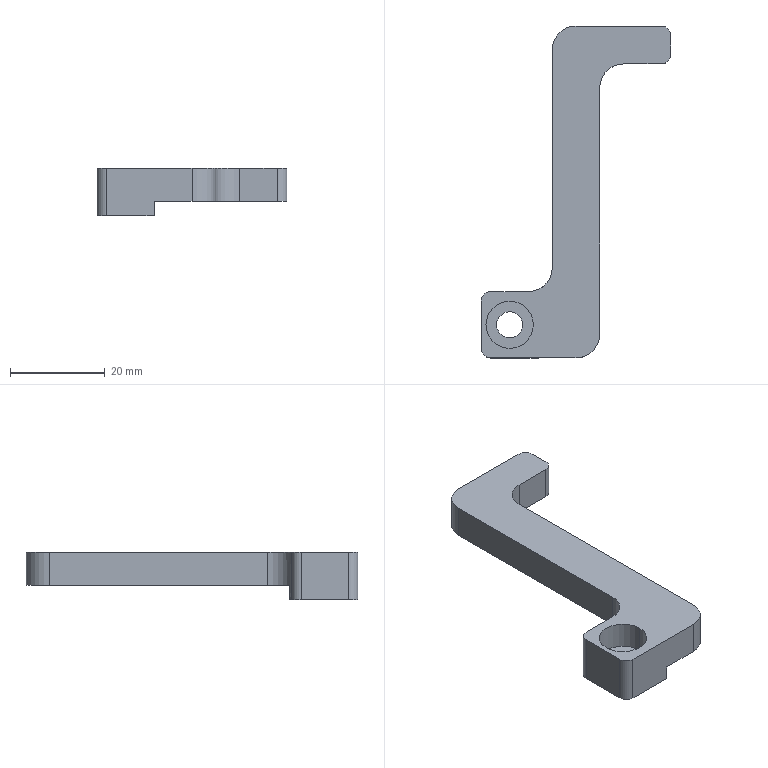Part | STEP file | FBDS-CS-027 | 1 solid | 34 faces | box 40 x 70 x 10 mm | volume 7093 mm3 | plane 18 | cylinder 16 | commonest cylinder face diameters 10 x6 4 x4 8 x4 5.5 x2
STEP:
#1=CARTESIAN_POINT('',(-14.,7.,4.3));
#2=VERTEX_POINT('',#1);
#3=CARTESIAN_POINT('',(-4.,7.,4.3));
#4=VERTEX_POINT('',#3);
#5=CARTESIAN_POINT('',(-9.,7.,4.3));
#6=DIRECTION('',(0.,0.,1.));
#7=DIRECTION('',(1.,0.,0.));
#8=AXIS2_PLACEMENT_3D('',#5,#6,#7);
#9=CIRCLE('',#8,5.);
#10=EDGE_CURVE('',#2,#4,#9,.T.);
#11=ORIENTED_EDGE('',*,*,#10,.F.);
#12=CARTESIAN_POINT('',(-14.,7.,10.));
#13=VERTEX_POINT('',#12);
#14=CARTESIAN_POINT('',(-14.,7.,10.));
#15=DIRECTION('',(0.,0.,1.));
#16=VECTOR('',#15,1000.);
#17=LINE('',#14,#16);
#18=EDGE_CURVE('',#2,#13,#17,.T.);
#19=ORIENTED_EDGE('',*,*,#18,.T.);
#20=CARTESIAN_POINT('',(-4.,7.,10.));
#21=VERTEX_POINT('',#20);
#22=CARTESIAN_POINT('',(-9.,7.,10.));
#23=DIRECTION('',(0.,0.,1.));
#24=DIRECTION('',(1.,0.,0.));
#25=AXIS2_PLACEMENT_3D('',#22,#23,#24);
#26=CIRCLE('',#25,5.);
#27=EDGE_CURVE('',#13,#21,#26,.T.);
#28=ORIENTED_EDGE('',*,*,#27,.T.);
#29=CARTESIAN_POINT('',(-4.,7.,10.));
#30=DIRECTION('',(0.,0.,1.));
#31=VECTOR('',#30,1000.);
#32=LINE('',#29,#31);
#33=EDGE_CURVE('',#4,#21,#32,.T.);
#34=ORIENTED_EDGE('',*,*,#33,.F.);
#35=EDGE_LOOP('',(#11,#19,#28,#34));
#36=FACE_OUTER_BOUND('',#35,.T.);
#37=CARTESIAN_POINT('',(-9.,7.,10.));
#38=DIRECTION('',(0.,0.,1.));
#39=DIRECTION('',(1.,0.,0.));
#40=AXIS2_PLACEMENT_3D('',#37,#38,#39);
#41=CYLINDRICAL_SURFACE('',#40,5.);
#42=ADVANCED_FACE('',(#36),#41,.F.);
#43=CARTESIAN_POINT('',(-6.25,7.,2.));
#44=VERTEX_POINT('',#43);
#45=CARTESIAN_POINT('',(-11.75,7.,2.));
#46=VERTEX_POINT('',#45);
#47=CARTESIAN_POINT('',(-9.,7.,2.));
#48=DIRECTION('',(0.,0.,-1.));
#49=DIRECTION('',(-1.,0.,0.));
#50=AXIS2_PLACEMENT_3D('',#47,#48,#49);
#51=CIRCLE('',#50,2.75);
#52=EDGE_CURVE('',#44,#46,#51,.T.);
#53=ORIENTED_EDGE('',*,*,#52,.T.);
#54=CARTESIAN_POINT('',(-11.75,7.,4.3));
#55=VERTEX_POINT('',#54);
#56=CARTESIAN_POINT('',(-11.75,7.,10.));
#57=DIRECTION('',(0.,0.,1.));
#58=VECTOR('',#57,1000.);
#59=LINE('',#56,#58);
#60=EDGE_CURVE('',#46,#55,#59,.T.);
#61=ORIENTED_EDGE('',*,*,#60,.T.);
#62=CARTESIAN_POINT('',(-6.25,7.,4.3));
#63=VERTEX_POINT('',#62);
#64=CARTESIAN_POINT('',(-9.,7.,4.3));
#65=DIRECTION('',(0.,0.,1.));
#66=DIRECTION('',(1.,0.,0.));
#67=AXIS2_PLACEMENT_3D('',#64,#65,#66);
#68=CIRCLE('',#67,2.75);
#69=EDGE_CURVE('',#55,#63,#68,.T.);
#70=ORIENTED_EDGE('',*,*,#69,.T.);
#71=CARTESIAN_POINT('',(-6.25,7.,10.));
#72=DIRECTION('',(0.,0.,1.));
#73=VECTOR('',#72,1000.);
#74=LINE('',#71,#73);
#75=EDGE_CURVE('',#44,#63,#74,.T.);
#76=ORIENTED_EDGE('',*,*,#75,.F.);
#77=EDGE_LOOP('',(#53,#61,#70,#76));
#78=FACE_OUTER_BOUND('',#77,.T.);
#79=CARTESIAN_POINT('',(-9.,7.,10.));
#80=DIRECTION('',(0.,0.,1.));
#81=DIRECTION('',(1.,0.,0.));
#82=AXIS2_PLACEMENT_3D('',#79,#80,#81);
#83=CYLINDRICAL_SURFACE('',#82,2.75);
#84=ADVANCED_FACE('',(#78),#83,.F.);
#85=CARTESIAN_POINT('',(0.,19.,3.));
#86=VERTEX_POINT('',#85);
#87=CARTESIAN_POINT('',(0.,65.,3.));
#88=VERTEX_POINT('',#87);
#89=CARTESIAN_POINT('',(0.,70.,3.));
#90=DIRECTION('',(0.,1.,0.));
#91=VECTOR('',#90,1000.);
#92=LINE('',#89,#91);
#93=EDGE_CURVE('',#86,#88,#92,.T.);
#94=ORIENTED_EDGE('',*,*,#93,.F.);
#95=CARTESIAN_POINT('',(0.,19.,10.));
#96=VERTEX_POINT('',#95);
#97=CARTESIAN_POINT('',(0.,19.,10.));
#98=DIRECTION('',(0.,0.,1.));
#99=VECTOR('',#98,1000.);
#100=LINE('',#97,#99);
#101=EDGE_CURVE('',#86,#96,#100,.T.);
#102=ORIENTED_EDGE('',*,*,#101,.T.);
#103=CARTESIAN_POINT('',(0.,65.,10.));
#104=VERTEX_POINT('',#103);
#105=CARTESIAN_POINT('',(0.,70.,10.));
#106=DIRECTION('',(0.,-1.,0.));
#107=VECTOR('',#106,1000.);
#108=LINE('',#105,#107);
#109=EDGE_CURVE('',#104,#96,#108,.T.);
#110=ORIENTED_EDGE('',*,*,#109,.F.);
#111=CARTESIAN_POINT('',(0.,65.,10.));
#112=DIRECTION('',(0.,0.,-1.));
#113=VECTOR('',#112,1000.);
#114=LINE('',#111,#113);
#115=EDGE_CURVE('',#104,#88,#114,.T.);
#116=ORIENTED_EDGE('',*,*,#115,.T.);
#117=EDGE_LOOP('',(#94,#102,#110,#116));
#118=FACE_OUTER_BOUND('',#117,.T.);
#119=CARTESIAN_POINT('',(0.,70.,10.));
#120=DIRECTION('',(1.,0.,0.));
#121=DIRECTION('',(0.,1.,0.));
#122=AXIS2_PLACEMENT_3D('',#119,#120,#121);
#123=PLANE('',#122);
#124=ADVANCED_FACE('',(#118),#123,.F.);
#125=CARTESIAN_POINT('',(10.,57.,3.));
#126=VERTEX_POINT('',#125);
#127=CARTESIAN_POINT('',(10.,5.,3.));
#128=VERTEX_POINT('',#127);
#129=CARTESIAN_POINT('',(10.,0.,3.));
#130=DIRECTION('',(0.,-1.,0.));
#131=VECTOR('',#130,1000.);
#132=LINE('',#129,#131);
#133=EDGE_CURVE('',#126,#128,#132,.T.);
#134=ORIENTED_EDGE('',*,*,#133,.F.);
#135=CARTESIAN_POINT('',(10.,57.,10.));
#136=VERTEX_POINT('',#135);
#137=CARTESIAN_POINT('',(10.,57.,10.));
#138=DIRECTION('',(0.,0.,1.));
#139=VECTOR('',#138,1000.);
#140=LINE('',#137,#139);
#141=EDGE_CURVE('',#126,#136,#140,.T.);
#142=ORIENTED_EDGE('',*,*,#141,.T.);
#143=CARTESIAN_POINT('',(10.,5.,10.));
#144=VERTEX_POINT('',#143);
#145=CARTESIAN_POINT('',(10.,0.,10.));
#146=DIRECTION('',(0.,1.,0.));
#147=VECTOR('',#146,1000.);
#148=LINE('',#145,#147);
#149=EDGE_CURVE('',#144,#136,#148,.T.);
#150=ORIENTED_EDGE('',*,*,#149,.F.);
#151=CARTESIAN_POINT('',(10.,5.,10.));
#152=DIRECTION('',(0.,0.,-1.));
#153=VECTOR('',#152,1000.);
#154=LINE('',#151,#153);
#155=EDGE_CURVE('',#144,#128,#154,.T.);
#156=ORIENTED_EDGE('',*,*,#155,.T.);
#157=EDGE_LOOP('',(#134,#142,#150,#156));
#158=FACE_OUTER_BOUND('',#157,.T.);
#159=CARTESIAN_POINT('',(10.,0.,10.));
#160=DIRECTION('',(-1.,0.,0.));
#161=DIRECTION('',(0.,0.,1.));
#162=AXIS2_PLACEMENT_3D('',#159,#160,#161);
#163=PLANE('',#162);
#164=ADVANCED_FACE('',(#158),#163,.F.);
#165=CARTESIAN_POINT('',(23.,62.,3.));
#166=VERTEX_POINT('',#165);
#167=CARTESIAN_POINT('',(15.,62.,3.));
#168=VERTEX_POINT('',#167);
#169=CARTESIAN_POINT('',(10.,62.,3.));
#170=DIRECTION('',(-1.,0.,0.));
#171=VECTOR('',#170,1000.);
#172=LINE('',#169,#171);
#173=EDGE_CURVE('',#166,#168,#172,.T.);
#174=ORIENTED_EDGE('',*,*,#173,.F.);
#175=CARTESIAN_POINT('',(23.,62.,10.));
#176=VERTEX_POINT('',#175);
#177=CARTESIAN_POINT('',(23.,62.,10.));
#178=DIRECTION('',(0.,0.,1.));
#179=VECTOR('',#178,1000.);
#180=LINE('',#177,#179);
#181=EDGE_CURVE('',#166,#176,#180,.T.);
#182=ORIENTED_EDGE('',*,*,#181,.T.);
#183=CARTESIAN_POINT('',(15.,62.,10.));
#184=VERTEX_POINT('',#183);
#185=CARTESIAN_POINT('',(10.,62.,10.));
#186=DIRECTION('',(1.,0.,0.));
#187=VECTOR('',#186,1000.);
#188=LINE('',#185,#187);
#189=EDGE_CURVE('',#184,#176,#188,.T.);
#190=ORIENTED_EDGE('',*,*,#189,.F.);
#191=CARTESIAN_POINT('',(15.,62.,0.));
#192=DIRECTION('',(0.,0.,-1.));
#193=VECTOR('',#192,1000.);
#194=LINE('',#191,#193);
#195=EDGE_CURVE('',#184,#168,#194,.T.);
#196=ORIENTED_EDGE('',*,*,#195,.T.);
#197=EDGE_LOOP('',(#174,#182,#190,#196));
#198=FACE_OUTER_BOUND('',#197,.T.);
#199=CARTESIAN_POINT('',(10.,62.,10.));
#200=DIRECTION('',(0.,1.,0.));
#201=DIRECTION('',(0.,0.,1.));
#202=AXIS2_PLACEMENT_3D('',#199,#200,#201);
#203=PLANE('',#202);
#204=ADVANCED_FACE('',(#198),#203,.F.);
#205=CARTESIAN_POINT('',(25.,64.,10.));
#206=VERTEX_POINT('',#205);
#207=CARTESIAN_POINT('',(25.,68.,10.));
#208=VERTEX_POINT('',#207);
#209=CARTESIAN_POINT('',(25.,62.,10.));
#210=DIRECTION('',(0.,1.,0.));
#211=VECTOR('',#210,1000.);
#212=LINE('',#209,#211);
#213=EDGE_CURVE('',#206,#208,#212,.T.);
#214=ORIENTED_EDGE('',*,*,#213,.F.);
#215=CARTESIAN_POINT('',(25.,64.,3.));
#216=VERTEX_POINT('',#215);
#217=CARTESIAN_POINT('',(25.,64.,10.));
#218=DIRECTION('',(0.,0.,-1.));
#219=VECTOR('',#218,1000.);
#220=LINE('',#217,#219);
#221=EDGE_CURVE('',#206,#216,#220,.T.);
#222=ORIENTED_EDGE('',*,*,#221,.T.);
#223=CARTESIAN_POINT('',(25.,68.,3.));
#224=VERTEX_POINT('',#223);
#225=CARTESIAN_POINT('',(25.,70.,3.));
#226=DIRECTION('',(0.,-1.,0.));
#227=VECTOR('',#226,1000.);
#228=LINE('',#225,#227);
#229=EDGE_CURVE('',#224,#216,#228,.T.);
#230=ORIENTED_EDGE('',*,*,#229,.F.);
#231=CARTESIAN_POINT('',(25.,68.,10.));
#232=DIRECTION('',(0.,0.,1.));
#233=VECTOR('',#232,1000.);
#234=LINE('',#231,#233);
#235=EDGE_CURVE('',#224,#208,#234,.T.);
#236=ORIENTED_EDGE('',*,*,#235,.T.);
#237=EDGE_LOOP('',(#214,#222,#230,#236));
#238=FACE_OUTER_BOUND('',#237,.T.);
#239=CARTESIAN_POINT('',(25.,62.,10.));
#240=DIRECTION('',(-1.,0.,0.));
#241=DIRECTION('',(0.,0.,1.));
#242=AXIS2_PLACEMENT_3D('',#239,#240,#241);
#243=PLANE('',#242);
#244=ADVANCED_FACE('',(#238),#243,.F.);
#245=CARTESIAN_POINT('',(23.,70.,10.));
#246=VERTEX_POINT('',#245);
#247=CARTESIAN_POINT('',(5.,70.,10.));
#248=VERTEX_POINT('',#247);
#249=CARTESIAN_POINT('',(25.,70.,10.));
#250=DIRECTION('',(-1.,0.,0.));
#251=VECTOR('',#250,1000.);
#252=LINE('',#249,#251);
#253=EDGE_CURVE('',#246,#248,#252,.T.);
#254=ORIENTED_EDGE('',*,*,#253,.F.);
#255=CARTESIAN_POINT('',(23.,70.,3.));
#256=VERTEX_POINT('',#255);
#257=CARTESIAN_POINT('',(23.,70.,10.));
#258=DIRECTION('',(0.,0.,-1.));
#259=VECTOR('',#258,1000.);
#260=LINE('',#257,#259);
#261=EDGE_CURVE('',#246,#256,#260,.T.);
#262=ORIENTED_EDGE('',*,*,#261,.T.);
#263=CARTESIAN_POINT('',(5.,70.,3.));
#264=VERTEX_POINT('',#263);
#265=CARTESIAN_POINT('',(25.,70.,3.));
#266=DIRECTION('',(1.,0.,0.));
#267=VECTOR('',#266,1000.);
#268=LINE('',#265,#267);
#269=EDGE_CURVE('',#264,#256,#268,.T.);
#270=ORIENTED_EDGE('',*,*,#269,.F.);
#271=CARTESIAN_POINT('',(5.,70.,10.));
#272=DIRECTION('',(0.,0.,1.));
#273=VECTOR('',#272,1000.);
#274=LINE('',#271,#273);
#275=EDGE_CURVE('',#264,#248,#274,.T.);
#276=ORIENTED_EDGE('',*,*,#275,.T.);
#277=EDGE_LOOP('',(#254,#262,#270,#276));
#278=FACE_OUTER_BOUND('',#277,.T.);
#279=CARTESIAN_POINT('',(25.,70.,10.));
#280=DIRECTION('',(0.,-1.,0.));
#281=DIRECTION('',(0.,0.,-1.));
#282=AXIS2_PLACEMENT_3D('',#279,#280,#281);
#283=PLANE('',#282);
#284=ADVANCED_FACE('',(#278),#283,.F.);
#285=ORIENTED_EDGE('',*,*,#275,.F.);
#286=CARTESIAN_POINT('',(5.,65.,3.));
#287=DIRECTION('',(0.,0.,1.));
#288=DIRECTION('',(-1.,0.,0.));
#289=AXIS2_PLACEMENT_3D('',#286,#287,#288);
#290=CIRCLE('',#289,5.);
#291=EDGE_CURVE('',#264,#88,#290,.T.);
#292=ORIENTED_EDGE('',*,*,#291,.T.);
#293=ORIENTED_EDGE('',*,*,#115,.F.);
#294=CARTESIAN_POINT('',(5.,65.,10.));
#295=DIRECTION('',(0.,0.,1.));
#296=DIRECTION('',(1.,0.,0.));
#297=AXIS2_PLACEMENT_3D('',#294,#295,#296);
#298=CIRCLE('',#297,5.);
#299=EDGE_CURVE('',#248,#104,#298,.T.);
#300=ORIENTED_EDGE('',*,*,#299,.F.);
#301=EDGE_LOOP('',(#285,#292,#293,#300));
#302=FACE_OUTER_BOUND('',#301,.T.);
#303=CARTESIAN_POINT('',(5.,65.,10.));
#304=DIRECTION('',(0.,0.,-1.));
#305=DIRECTION('',(-1.,0.,0.));
#306=AXIS2_PLACEMENT_3D('',#303,#304,#305);
#307=CYLINDRICAL_SURFACE('',#306,5.);
#308=ADVANCED_FACE('',(#302),#307,.T.);
#309=CARTESIAN_POINT('',(5.,0.,3.));
#310=VERTEX_POINT('',#309);
#311=CARTESIAN_POINT('',(5.,0.,10.));
#312=VERTEX_POINT('',#311);
#313=CARTESIAN_POINT('',(5.,0.,10.));
#314=DIRECTION('',(0.,0.,1.));
#315=VECTOR('',#314,1000.);
#316=LINE('',#313,#315);
#317=EDGE_CURVE('',#310,#312,#316,.T.);
#318=ORIENTED_EDGE('',*,*,#317,.F.);
#319=CARTESIAN_POINT('',(5.,5.,3.));
#320=DIRECTION('',(0.,0.,1.));
#321=DIRECTION('',(-1.,0.,0.));
#322=AXIS2_PLACEMENT_3D('',#319,#320,#321);
#323=CIRCLE('',#322,5.);
#324=EDGE_CURVE('',#310,#128,#323,.T.);
#325=ORIENTED_EDGE('',*,*,#324,.T.);
#326=ORIENTED_EDGE('',*,*,#155,.F.);
#327=CARTESIAN_POINT('',(5.,5.,10.));
#328=DIRECTION('',(0.,0.,1.));
#329=DIRECTION('',(1.,0.,0.));
#330=AXIS2_PLACEMENT_3D('',#327,#328,#329);
#331=CIRCLE('',#330,5.);
#332=EDGE_CURVE('',#312,#144,#331,.T.);
#333=ORIENTED_EDGE('',*,*,#332,.F.);
#334=EDGE_LOOP('',(#318,#325,#326,#333));
#335=FACE_OUTER_BOUND('',#334,.T.);
#336=CARTESIAN_POINT('',(5.,5.,10.));
#337=DIRECTION('',(0.,0.,-1.));
#338=DIRECTION('',(-1.,0.,0.));
#339=AXIS2_PLACEMENT_3D('',#336,#337,#338);
#340=CYLINDRICAL_SURFACE('',#339,5.);
#341=ADVANCED_FACE('',(#335),#340,.T.);
#342=CARTESIAN_POINT('',(15.,57.,3.));
#343=DIRECTION('',(0.,0.,1.));
#344=DIRECTION('',(-1.,0.,0.));
#345=AXIS2_PLACEMENT_3D('',#342,#343,#344);
#346=CIRCLE('',#345,5.);
#347=EDGE_CURVE('',#168,#126,#346,.T.);
#348=ORIENTED_EDGE('',*,*,#347,.F.);
#349=ORIENTED_EDGE('',*,*,#195,.F.);
#350=CARTESIAN_POINT('',(15.,57.,10.));
#351=DIRECTION('',(0.,0.,-1.));
#352=DIRECTION('',(1.,0.,0.));
#353=AXIS2_PLACEMENT_3D('',#350,#351,#352);
#354=CIRCLE('',#353,5.);
#355=EDGE_CURVE('',#136,#184,#354,.T.);
#356=ORIENTED_EDGE('',*,*,#355,.F.);
#357=ORIENTED_EDGE('',*,*,#141,.F.);
#358=EDGE_LOOP('',(#348,#349,#356,#357));
#359=FACE_OUTER_BOUND('',#358,.T.);
#360=CARTESIAN_POINT('',(15.,57.,10.));
#361=DIRECTION('',(0.,0.,1.));
#362=DIRECTION('',(1.,0.,0.));
#363=AXIS2_PLACEMENT_3D('',#360,#361,#362);
#364=CYLINDRICAL_SURFACE('',#363,5.);
#365=ADVANCED_FACE('',(#359),#364,.F.);
#366=CARTESIAN_POINT('',(-13.,0.,10.));
#367=VERTEX_POINT('',#366);
#368=CARTESIAN_POINT('',(0.,0.,10.));
#369=DIRECTION('',(1.,0.,0.));
#370=VECTOR('',#369,1000.);
#371=LINE('',#368,#370);
#372=EDGE_CURVE('',#367,#312,#371,.T.);
#373=ORIENTED_EDGE('',*,*,#372,.F.);
#374=CARTESIAN_POINT('',(-13.,0.,0.));
#375=VERTEX_POINT('',#374);
#376=CARTESIAN_POINT('',(-13.,0.,0.));
#377=DIRECTION('',(0.,0.,-1.));
#378=VECTOR('',#377,1000.);
#379=LINE('',#376,#378);
#380=EDGE_CURVE('',#367,#375,#379,.T.);
#381=ORIENTED_EDGE('',*,*,#380,.T.);
#382=CARTESIAN_POINT('',(-3.,0.,0.));
#383=VERTEX_POINT('',#382);
#384=CARTESIAN_POINT('',(0.,0.,0.));
#385=DIRECTION('',(1.,0.,0.));
#386=VECTOR('',#385,1000.);
#387=LINE('',#384,#386);
#388=EDGE_CURVE('',#375,#383,#387,.T.);
#389=ORIENTED_EDGE('',*,*,#388,.T.);
#390=CARTESIAN_POINT('',(-3.,0.,3.));
#391=VERTEX_POINT('',#390);
#392=CARTESIAN_POINT('',(-3.,0.,10.));
#393=DIRECTION('',(0.,0.,1.));
#394=VECTOR('',#393,1000.);
#395=LINE('',#392,#394);
#396=EDGE_CURVE('',#383,#391,#395,.T.);
#397=ORIENTED_EDGE('',*,*,#396,.T.);
#398=CARTESIAN_POINT('',(0.,0.,3.));
#399=DIRECTION('',(-1.,0.,0.));
#400=VECTOR('',#399,1000.);
#401=LINE('',#398,#400);
#402=EDGE_CURVE('',#310,#391,#401,.T.);
#403=ORIENTED_EDGE('',*,*,#402,.F.);
#404=ORIENTED_EDGE('',*,*,#317,.T.);
#405=EDGE_LOOP('',(#373,#381,#389,#397,#403,#404));
#406=FACE_OUTER_BOUND('',#405,.T.);
#407=CARTESIAN_POINT('',(0.,0.,10.));
#408=DIRECTION('',(0.,1.,0.));
#409=DIRECTION('',(0.,0.,1.));
#410=AXIS2_PLACEMENT_3D('',#407,#408,#409);
#411=PLANE('',#410);
#412=ADVANCED_FACE('',(#406),#411,.F.);
#413=CARTESIAN_POINT('',(-9.,7.,10.));
#414=DIRECTION('',(0.,0.,1.));
#415=DIRECTION('',(1.,0.,0.));
#416=AXIS2_PLACEMENT_3D('',#413,#414,#415);
#417=CIRCLE('',#416,5.);
#418=EDGE_CURVE('',#21,#13,#417,.T.);
#419=ORIENTED_EDGE('',*,*,#418,.F.);
#420=ORIENTED_EDGE('',*,*,#27,.F.);
#421=EDGE_LOOP('',(#419,#420));
#422=FACE_BOUND('',#421,.T.);
#423=ORIENTED_EDGE('',*,*,#189,.T.);
#424=CARTESIAN_POINT('',(23.,64.,10.));
#425=DIRECTION('',(0.,0.,1.));
#426=DIRECTION('',(1.,0.,0.));
#427=AXIS2_PLACEMENT_3D('',#424,#425,#426);
#428=CIRCLE('',#427,2.);
#429=EDGE_CURVE('',#176,#206,#428,.T.);
#430=ORIENTED_EDGE('',*,*,#429,.T.);
#431=ORIENTED_EDGE('',*,*,#213,.T.);
#432=CARTESIAN_POINT('',(23.,68.,10.));
#433=DIRECTION('',(0.,0.,1.));
#434=DIRECTION('',(1.,0.,0.));
#435=AXIS2_PLACEMENT_3D('',#432,#433,#434);
#436=CIRCLE('',#435,2.);
#437=EDGE_CURVE('',#208,#246,#436,.T.);
#438=ORIENTED_EDGE('',*,*,#437,.T.);
#439=ORIENTED_EDGE('',*,*,#253,.T.);
#440=ORIENTED_EDGE('',*,*,#299,.T.);
#441=ORIENTED_EDGE('',*,*,#109,.T.);
#442=CARTESIAN_POINT('',(-5.,14.,10.));
#443=VERTEX_POINT('',#442);
#444=CARTESIAN_POINT('',(-5.,19.,10.));
#445=DIRECTION('',(0.,0.,-1.));
#446=DIRECTION('',(1.,0.,0.));
#447=AXIS2_PLACEMENT_3D('',#444,#445,#446);
#448=CIRCLE('',#447,5.);
#449=EDGE_CURVE('',#96,#443,#448,.T.);
#450=ORIENTED_EDGE('',*,*,#449,.T.);
#451=CARTESIAN_POINT('',(-13.,14.,10.));
#452=VERTEX_POINT('',#451);
#453=CARTESIAN_POINT('',(0.,14.,10.));
#454=DIRECTION('',(-1.,0.,0.));
#455=VECTOR('',#454,1000.);
#456=LINE('',#453,#455);
#457=EDGE_CURVE('',#443,#452,#456,.T.);
#458=ORIENTED_EDGE('',*,*,#457,.T.);
#459=CARTESIAN_POINT('',(-15.,12.,10.));
#460=VERTEX_POINT('',#459);
#461=CARTESIAN_POINT('',(-13.,12.,10.));
#462=DIRECTION('',(0.,0.,1.));
#463=DIRECTION('',(1.,0.,0.));
#464=AXIS2_PLACEMENT_3D('',#461,#462,#463);
#465=CIRCLE('',#464,2.);
#466=EDGE_CURVE('',#452,#460,#465,.T.);
#467=ORIENTED_EDGE('',*,*,#466,.T.);
#468=CARTESIAN_POINT('',(-15.,2.,10.));
#469=VERTEX_POINT('',#468);
#470=CARTESIAN_POINT('',(-15.,0.,10.));
#471=DIRECTION('',(0.,-1.,0.));
#472=VECTOR('',#471,1000.);
#473=LINE('',#470,#472);
#474=EDGE_CURVE('',#460,#469,#473,.T.);
#475=ORIENTED_EDGE('',*,*,#474,.T.);
#476=CARTESIAN_POINT('',(-13.,2.,10.));
#477=DIRECTION('',(0.,0.,1.));
#478=DIRECTION('',(1.,0.,0.));
#479=AXIS2_PLACEMENT_3D('',#476,#477,#478);
#480=CIRCLE('',#479,2.);
#481=EDGE_CURVE('',#469,#367,#480,.T.);
#482=ORIENTED_EDGE('',*,*,#481,.T.);
#483=ORIENTED_EDGE('',*,*,#372,.T.);
#484=ORIENTED_EDGE('',*,*,#332,.T.);
#485=ORIENTED_EDGE('',*,*,#149,.T.);
#486=ORIENTED_EDGE('',*,*,#355,.T.);
#487=EDGE_LOOP('',(#423,#430,#431,#438,#439,#440,#441,#450,#458,#467,#475,#482,#483,#484,#485,#486));
#488=FACE_OUTER_BOUND('',#487,.T.);
#489=CARTESIAN_POINT('',(0.,0.,10.));
#490=DIRECTION('',(0.,0.,1.));
#491=DIRECTION('',(1.,0.,0.));
#492=AXIS2_PLACEMENT_3D('',#489,#490,#491);
#493=PLANE('',#492);
#494=ADVANCED_FACE('',(#422,#488),#493,.T.);
#495=CARTESIAN_POINT('',(-10.936,10.5,0.));
#496=VERTEX_POINT('',#495);
#497=CARTESIAN_POINT('',(-7.064,10.5,0.));
#498=VERTEX_POINT('',#497);
#499=CARTESIAN_POINT('',(-7.064,10.5,0.));
#500=DIRECTION('',(1.,0.,0.));
#501=VECTOR('',#500,1000.);
#502=LINE('',#499,#501);
#503=EDGE_CURVE('',#496,#498,#502,.T.);
#504=ORIENTED_EDGE('',*,*,#503,.F.);
#505=CARTESIAN_POINT('',(-12.5,8.936,0.));
#506=VERTEX_POINT('',#505);
#507=CARTESIAN_POINT('',(-9.,7.,0.));
#508=DIRECTION('',(0.,0.,-1.));
#509=DIRECTION('',(-1.,0.,0.));
#510=AXIS2_PLACEMENT_3D('',#507,#508,#509);
#511=CIRCLE('',#510,4.);
#512=EDGE_CURVE('',#506,#496,#511,.T.);
#513=ORIENTED_EDGE('',*,*,#512,.F.);
#514=CARTESIAN_POINT('',(-12.5,5.064,0.));
#515=VERTEX_POINT('',#514);
#516=CARTESIAN_POINT('',(-12.5,5.064,0.));
#517=DIRECTION('',(0.,1.,0.));
#518=VECTOR('',#517,1000.);
#519=LINE('',#516,#518);
#520=EDGE_CURVE('',#515,#506,#519,.T.);
#521=ORIENTED_EDGE('',*,*,#520,.F.);
#522=CARTESIAN_POINT('',(-10.936,3.5,0.));
#523=VERTEX_POINT('',#522);
#524=CARTESIAN_POINT('',(-9.,7.,0.));
#525=DIRECTION('',(0.,0.,-1.));
#526=DIRECTION('',(-1.,0.,0.));
#527=AXIS2_PLACEMENT_3D('',#524,#525,#526);
#528=CIRCLE('',#527,4.);
#529=EDGE_CURVE('',#523,#515,#528,.T.);
#530=ORIENTED_EDGE('',*,*,#529,.F.);
#531=CARTESIAN_POINT('',(-7.064,3.5,0.));
#532=VERTEX_POINT('',#531);
#533=CARTESIAN_POINT('',(-7.064,3.5,0.));
#534=DIRECTION('',(-1.,0.,0.));
#535=VECTOR('',#534,1000.);
#536=LINE('',#533,#535);
#537=EDGE_CURVE('',#532,#523,#536,.T.);
#538=ORIENTED_EDGE('',*,*,#537,.F.);
#539=CARTESIAN_POINT('',(-5.5,5.064,0.));
#540=VERTEX_POINT('',#539);
#541=CARTESIAN_POINT('',(-9.,7.,0.));
#542=DIRECTION('',(0.,0.,-1.));
#543=DIRECTION('',(-1.,0.,0.));
#544=AXIS2_PLACEMENT_3D('',#541,#542,#543);
#545=CIRCLE('',#544,4.);
#546=EDGE_CURVE('',#540,#532,#545,.T.);
#547=ORIENTED_EDGE('',*,*,#546,.F.);
#548=CARTESIAN_POINT('',(-5.5,8.936,0.));
#549=VERTEX_POINT('',#548);
#550=CARTESIAN_POINT('',(-5.5,5.064,0.));
#551=DIRECTION('',(0.,-1.,0.));
#552=VECTOR('',#551,1000.);
#553=LINE('',#550,#552);
#554=EDGE_CURVE('',#549,#540,#553,.T.);
#555=ORIENTED_EDGE('',*,*,#554,.F.);
#556=CARTESIAN_POINT('',(-9.,7.,0.));
#557=DIRECTION('',(0.,0.,-1.));
#558=DIRECTION('',(-1.,0.,0.));
#559=AXIS2_PLACEMENT_3D('',#556,#557,#558);
#560=CIRCLE('',#559,4.);
#561=EDGE_CURVE('',#498,#549,#560,.T.);
#562=ORIENTED_EDGE('',*,*,#561,.F.);
#563=EDGE_LOOP('',(#504,#513,#521,#530,#538,#547,#555,#562));
#564=FACE_BOUND('',#563,.T.);
#565=ORIENTED_EDGE('',*,*,#388,.F.);
#566=CARTESIAN_POINT('',(-15.,2.,0.));
#567=VERTEX_POINT('',#566);
#568=CARTESIAN_POINT('',(-13.,2.,0.));
#569=DIRECTION('',(0.,0.,-1.));
#570=DIRECTION('',(1.,0.,0.));
#571=AXIS2_PLACEMENT_3D('',#568,#569,#570);
#572=CIRCLE('',#571,2.);
#573=EDGE_CURVE('',#375,#567,#572,.T.);
#574=ORIENTED_EDGE('',*,*,#573,.T.);
#575=CARTESIAN_POINT('',(-15.,12.,0.));
#576=VERTEX_POINT('',#575);
#577=CARTESIAN_POINT('',(-15.,0.,0.));
#578=DIRECTION('',(0.,1.,0.));
#579=VECTOR('',#578,1000.);
#580=LINE('',#577,#579);
#581=EDGE_CURVE('',#567,#576,#580,.T.);
#582=ORIENTED_EDGE('',*,*,#581,.T.);
#583=CARTESIAN_POINT('',(-13.,14.,0.));
#584=VERTEX_POINT('',#583);
#585=CARTESIAN_POINT('',(-13.,12.,0.));
#586=DIRECTION('',(0.,0.,-1.));
#587=DIRECTION('',(1.,0.,0.));
#588=AXIS2_PLACEMENT_3D('',#585,#586,#587);
#589=CIRCLE('',#588,2.);
#590=EDGE_CURVE('',#576,#584,#589,.T.);
#591=ORIENTED_EDGE('',*,*,#590,.T.);
#592=CARTESIAN_POINT('',(-5.,14.,0.));
#593=VERTEX_POINT('',#592);
#594=CARTESIAN_POINT('',(0.,14.,0.));
#595=DIRECTION('',(1.,0.,0.));
#596=VECTOR('',#595,1000.);
#597=LINE('',#594,#596);
#598=EDGE_CURVE('',#584,#593,#597,.T.);
#599=ORIENTED_EDGE('',*,*,#598,.T.);
#600=CARTESIAN_POINT('',(-3.,14.417,0.));
#601=VERTEX_POINT('',#600);
#602=CARTESIAN_POINT('',(-5.,19.,0.));
#603=DIRECTION('',(0.,0.,1.));
#604=DIRECTION('',(1.,0.,0.));
#605=AXIS2_PLACEMENT_3D('',#602,#603,#604);
#606=CIRCLE('',#605,5.);
#607=EDGE_CURVE('',#593,#601,#606,.T.);
#608=ORIENTED_EDGE('',*,*,#607,.T.);
#609=CARTESIAN_POINT('',(-3.,70.,0.));
#610=DIRECTION('',(0.,1.,0.));
#611=VECTOR('',#610,1000.);
#612=LINE('',#609,#611);
#613=EDGE_CURVE('',#383,#601,#612,.T.);
#614=ORIENTED_EDGE('',*,*,#613,.F.);
#615=EDGE_LOOP('',(#565,#574,#582,#591,#599,#608,#614));
#616=FACE_OUTER_BOUND('',#615,.T.);
#617=CARTESIAN_POINT('',(0.,0.,0.));
#618=DIRECTION('',(0.,0.,1.));
#619=DIRECTION('',(1.,0.,0.));
#620=AXIS2_PLACEMENT_3D('',#617,#618,#619);
#621=PLANE('',#620);
#622=ADVANCED_FACE('',(#564,#616),#621,.F.);
#623=ORIENTED_EDGE('',*,*,#581,.F.);
#624=CARTESIAN_POINT('',(-15.,2.,10.));
#625=DIRECTION('',(0.,0.,1.));
#626=VECTOR('',#625,1000.);
#627=LINE('',#624,#626);
#628=EDGE_CURVE('',#567,#469,#627,.T.);
#629=ORIENTED_EDGE('',*,*,#628,.T.);
#630=ORIENTED_EDGE('',*,*,#474,.F.);
#631=CARTESIAN_POINT('',(-15.,12.,-20.518));
#632=DIRECTION('',(0.,0.,-1.));
#633=VECTOR('',#632,1000.);
#634=LINE('',#631,#633);
#635=EDGE_CURVE('',#460,#576,#634,.T.);
#636=ORIENTED_EDGE('',*,*,#635,.T.);
#637=EDGE_LOOP('',(#623,#629,#630,#636));
#638=FACE_OUTER_BOUND('',#637,.T.);
#639=CARTESIAN_POINT('',(-15.,0.,-20.518));
#640=DIRECTION('',(-1.,0.,0.));
#641=DIRECTION('',(0.,0.,1.));
#642=AXIS2_PLACEMENT_3D('',#639,#640,#641);
#643=PLANE('',#642);
#644=ADVANCED_FACE('',(#638),#643,.T.);
#645=ORIENTED_EDGE('',*,*,#598,.F.);
#646=CARTESIAN_POINT('',(-13.,14.,-20.518));
#647=DIRECTION('',(0.,0.,1.));
#648=VECTOR('',#647,1000.);
#649=LINE('',#646,#648);
#650=EDGE_CURVE('',#584,#452,#649,.T.);
#651=ORIENTED_EDGE('',*,*,#650,.T.);
#652=ORIENTED_EDGE('',*,*,#457,.F.);
#653=CARTESIAN_POINT('',(-5.,14.,-20.518));
#654=DIRECTION('',(0.,0.,-1.));
#655=VECTOR('',#654,1000.);
#656=LINE('',#653,#655);
#657=EDGE_CURVE('',#443,#593,#656,.T.);
#658=ORIENTED_EDGE('',*,*,#657,.T.);
#659=EDGE_LOOP('',(#645,#651,#652,#658));
#660=FACE_OUTER_BOUND('',#659,.T.);
#661=CARTESIAN_POINT('',(0.,14.,-20.518));
#662=DIRECTION('',(0.,1.,0.));
#663=DIRECTION('',(-1.,0.,0.));
#664=AXIS2_PLACEMENT_3D('',#661,#662,#663);
#665=PLANE('',#664);
#666=ADVANCED_FACE('',(#660),#665,.T.);
#667=ORIENTED_EDGE('',*,*,#512,.T.);
#668=CARTESIAN_POINT('',(-10.936,10.5,2.));
#669=VERTEX_POINT('',#668);
#670=CARTESIAN_POINT('',(-10.936,10.5,2.));
#671=DIRECTION('',(0.,0.,-1.));
#672=VECTOR('',#671,1000.);
#673=LINE('',#670,#672);
#674=EDGE_CURVE('',#669,#496,#673,.T.);
#675=ORIENTED_EDGE('',*,*,#674,.F.);
#676=CARTESIAN_POINT('',(-12.5,8.936,2.));
#677=VERTEX_POINT('',#676);
#678=CARTESIAN_POINT('',(-9.,7.,2.));
#679=DIRECTION('',(0.,0.,-1.));
#680=DIRECTION('',(-1.,0.,0.));
#681=AXIS2_PLACEMENT_3D('',#678,#679,#680);
#682=CIRCLE('',#681,4.);
#683=EDGE_CURVE('',#677,#669,#682,.T.);
#684=ORIENTED_EDGE('',*,*,#683,.F.);
#685=CARTESIAN_POINT('',(-12.5,8.936,2.));
#686=DIRECTION('',(0.,0.,-1.));
#687=VECTOR('',#686,1000.);
#688=LINE('',#685,#687);
#689=EDGE_CURVE('',#677,#506,#688,.T.);
#690=ORIENTED_EDGE('',*,*,#689,.T.);
#691=EDGE_LOOP('',(#667,#675,#684,#690));
#692=FACE_OUTER_BOUND('',#691,.T.);
#693=CARTESIAN_POINT('',(-9.,7.,2.));
#694=DIRECTION('',(0.,0.,-1.));
#695=DIRECTION('',(-1.,0.,0.));
#696=AXIS2_PLACEMENT_3D('',#693,#694,#695);
#697=CYLINDRICAL_SURFACE('',#696,4.);
#698=ADVANCED_FACE('',(#692),#697,.F.);
#699=ORIENTED_EDGE('',*,*,#520,.T.);
#700=ORIENTED_EDGE('',*,*,#689,.F.);
#701=CARTESIAN_POINT('',(-12.5,5.064,2.));
#702=VERTEX_POINT('',#701);
#703=CARTESIAN_POINT('',(-12.5,5.064,2.));
#704=DIRECTION('',(0.,1.,0.));
#705=VECTOR('',#704,1000.);
#706=LINE('',#703,#705);
#707=EDGE_CURVE('',#702,#677,#706,.T.);
#708=ORIENTED_EDGE('',*,*,#707,.F.);
#709=CARTESIAN_POINT('',(-12.5,5.064,2.));
#710=DIRECTION('',(0.,0.,-1.));
#711=VECTOR('',#710,1000.);
#712=LINE('',#709,#711);
#713=EDGE_CURVE('',#702,#515,#712,.T.);
#714=ORIENTED_EDGE('',*,*,#713,.T.);
#715=EDGE_LOOP('',(#699,#700,#708,#714));
#716=FACE_OUTER_BOUND('',#715,.T.);
#717=CARTESIAN_POINT('',(-12.5,5.064,2.));
#718=DIRECTION('',(-1.,0.,0.));
#719=DIRECTION('',(0.,0.,1.));
#720=AXIS2_PLACEMENT_3D('',#717,#718,#719);
#721=PLANE('',#720);
#722=ADVANCED_FACE('',(#716),#721,.F.);
#723=ORIENTED_EDGE('',*,*,#529,.T.);
#724=ORIENTED_EDGE('',*,*,#713,.F.);
#725=CARTESIAN_POINT('',(-10.936,3.5,2.));
#726=VERTEX_POINT('',#725);
#727=CARTESIAN_POINT('',(-9.,7.,2.));
#728=DIRECTION('',(0.,0.,-1.));
#729=DIRECTION('',(-1.,0.,0.));
#730=AXIS2_PLACEMENT_3D('',#727,#728,#729);
#731=CIRCLE('',#730,4.);
#732=EDGE_CURVE('',#726,#702,#731,.T.);
#733=ORIENTED_EDGE('',*,*,#732,.F.);
#734=CARTESIAN_POINT('',(-10.936,3.5,2.));
#735=DIRECTION('',(0.,0.,-1.));
#736=VECTOR('',#735,1000.);
#737=LINE('',#734,#736);
#738=EDGE_CURVE('',#726,#523,#737,.T.);
#739=ORIENTED_EDGE('',*,*,#738,.T.);
#740=EDGE_LOOP('',(#723,#724,#733,#739));
#741=FACE_OUTER_BOUND('',#740,.T.);
#742=CARTESIAN_POINT('',(-9.,7.,2.));
#743=DIRECTION('',(0.,0.,-1.));
#744=DIRECTION('',(-1.,0.,0.));
#745=AXIS2_PLACEMENT_3D('',#742,#743,#744);
#746=CYLINDRICAL_SURFACE('',#745,4.);
#747=ADVANCED_FACE('',(#741),#746,.F.);
#748=ORIENTED_EDGE('',*,*,#537,.T.);
#749=ORIENTED_EDGE('',*,*,#738,.F.);
#750=CARTESIAN_POINT('',(-7.064,3.5,2.));
#751=VERTEX_POINT('',#750);
#752=CARTESIAN_POINT('',(-7.064,3.5,2.));
#753=DIRECTION('',(-1.,0.,0.));
#754=VECTOR('',#753,1000.);
#755=LINE('',#752,#754);
#756=EDGE_CURVE('',#751,#726,#755,.T.);
#757=ORIENTED_EDGE('',*,*,#756,.F.);
#758=CARTESIAN_POINT('',(-7.064,3.5,2.));
#759=DIRECTION('',(0.,0.,-1.));
#760=VECTOR('',#759,1000.);
#761=LINE('',#758,#760);
#762=EDGE_CURVE('',#751,#532,#761,.T.);
#763=ORIENTED_EDGE('',*,*,#762,.T.);
#764=EDGE_LOOP('',(#748,#749,#757,#763));
#765=FACE_OUTER_BOUND('',#764,.T.);
#766=CARTESIAN_POINT('',(-7.064,3.5,2.));
#767=DIRECTION('',(0.,-1.,0.));
#768=DIRECTION('',(0.,0.,-1.));
#769=AXIS2_PLACEMENT_3D('',#766,#767,#768);
#770=PLANE('',#769);
#771=ADVANCED_FACE('',(#765),#770,.F.);
#772=ORIENTED_EDGE('',*,*,#546,.T.);
#773=ORIENTED_EDGE('',*,*,#762,.F.);
#774=CARTESIAN_POINT('',(-5.5,5.064,2.));
#775=VERTEX_POINT('',#774);
#776=CARTESIAN_POINT('',(-9.,7.,2.));
#777=DIRECTION('',(0.,0.,-1.));
#778=DIRECTION('',(-1.,0.,0.));
#779=AXIS2_PLACEMENT_3D('',#776,#777,#778);
#780=CIRCLE('',#779,4.);
#781=EDGE_CURVE('',#775,#751,#780,.T.);
#782=ORIENTED_EDGE('',*,*,#781,.F.);
#783=CARTESIAN_POINT('',(-5.5,5.064,2.));
#784=DIRECTION('',(0.,0.,-1.));
#785=VECTOR('',#784,1000.);
#786=LINE('',#783,#785);
#787=EDGE_CURVE('',#775,#540,#786,.T.);
#788=ORIENTED_EDGE('',*,*,#787,.T.);
#789=EDGE_LOOP('',(#772,#773,#782,#788));
#790=FACE_OUTER_BOUND('',#789,.T.);
#791=CARTESIAN_POINT('',(-9.,7.,2.));
#792=DIRECTION('',(0.,0.,-1.));
#793=DIRECTION('',(-1.,0.,0.));
#794=AXIS2_PLACEMENT_3D('',#791,#792,#793);
#795=CYLINDRICAL_SURFACE('',#794,4.);
#796=ADVANCED_FACE('',(#790),#795,.F.);
#797=ORIENTED_EDGE('',*,*,#554,.T.);
#798=ORIENTED_EDGE('',*,*,#787,.F.);
#799=CARTESIAN_POINT('',(-5.5,8.936,2.));
#800=VERTEX_POINT('',#799);
#801=CARTESIAN_POINT('',(-5.5,5.064,2.));
#802=DIRECTION('',(0.,-1.,0.));
#803=VECTOR('',#802,1000.);
#804=LINE('',#801,#803);
#805=EDGE_CURVE('',#800,#775,#804,.T.);
#806=ORIENTED_EDGE('',*,*,#805,.F.);
#807=CARTESIAN_POINT('',(-5.5,8.936,2.));
#808=DIRECTION('',(0.,0.,-1.));
#809=VECTOR('',#808,1000.);
#810=LINE('',#807,#809);
#811=EDGE_CURVE('',#800,#549,#810,.T.);
#812=ORIENTED_EDGE('',*,*,#811,.T.);
#813=EDGE_LOOP('',(#797,#798,#806,#812));
#814=FACE_OUTER_BOUND('',#813,.T.);
#815=CARTESIAN_POINT('',(-5.5,5.064,2.));
#816=DIRECTION('',(1.,0.,0.));
#817=DIRECTION('',(0.,0.,-1.));
#818=AXIS2_PLACEMENT_3D('',#815,#816,#817);
#819=PLANE('',#818);
#820=ADVANCED_FACE('',(#814),#819,.F.);
#821=ORIENTED_EDGE('',*,*,#561,.T.);
#822=ORIENTED_EDGE('',*,*,#811,.F.);
#823=CARTESIAN_POINT('',(-7.064,10.5,2.));
#824=VERTEX_POINT('',#823);
#825=CARTESIAN_POINT('',(-9.,7.,2.));
#826=DIRECTION('',(0.,0.,-1.));
#827=DIRECTION('',(-1.,0.,0.));
#828=AXIS2_PLACEMENT_3D('',#825,#826,#827);
#829=CIRCLE('',#828,4.);
#830=EDGE_CURVE('',#824,#800,#829,.T.);
#831=ORIENTED_EDGE('',*,*,#830,.F.);
#832=CARTESIAN_POINT('',(-7.064,10.5,2.));
#833=DIRECTION('',(0.,0.,-1.));
#834=VECTOR('',#833,1000.);
#835=LINE('',#832,#834);
#836=EDGE_CURVE('',#824,#498,#835,.T.);
#837=ORIENTED_EDGE('',*,*,#836,.T.);
#838=EDGE_LOOP('',(#821,#822,#831,#837));
#839=FACE_OUTER_BOUND('',#838,.T.);
#840=CARTESIAN_POINT('',(-9.,7.,2.));
#841=DIRECTION('',(0.,0.,-1.));
#842=DIRECTION('',(-1.,0.,0.));
#843=AXIS2_PLACEMENT_3D('',#840,#841,#842);
#844=CYLINDRICAL_SURFACE('',#843,4.);
#845=ADVANCED_FACE('',(#839),#844,.F.);
#846=ORIENTED_EDGE('',*,*,#503,.T.);
#847=ORIENTED_EDGE('',*,*,#836,.F.);
#848=CARTESIAN_POINT('',(-7.064,10.5,2.));
#849=DIRECTION('',(1.,0.,0.));
#850=VECTOR('',#849,1000.);
#851=LINE('',#848,#850);
#852=EDGE_CURVE('',#669,#824,#851,.T.);
#853=ORIENTED_EDGE('',*,*,#852,.F.);
#854=ORIENTED_EDGE('',*,*,#674,.T.);
#855=EDGE_LOOP('',(#846,#847,#853,#854));
#856=FACE_OUTER_BOUND('',#855,.T.);
#857=CARTESIAN_POINT('',(-7.064,10.5,2.));
#858=DIRECTION('',(0.,1.,0.));
#859=DIRECTION('',(0.,0.,1.));
#860=AXIS2_PLACEMENT_3D('',#857,#858,#859);
#861=PLANE('',#860);
#862=ADVANCED_FACE('',(#856),#861,.F.);
#863=ORIENTED_EDGE('',*,*,#52,.F.);
#864=CARTESIAN_POINT('',(-9.,7.,2.));
#865=DIRECTION('',(0.,0.,-1.));
#866=DIRECTION('',(-1.,0.,0.));
#867=AXIS2_PLACEMENT_3D('',#864,#865,#866);
#868=CIRCLE('',#867,2.75);
#869=EDGE_CURVE('',#46,#44,#868,.T.);
#870=ORIENTED_EDGE('',*,*,#869,.F.);
#871=EDGE_LOOP('',(#863,#870));
#872=FACE_BOUND('',#871,.T.);
#873=ORIENTED_EDGE('',*,*,#683,.T.);
#874=ORIENTED_EDGE('',*,*,#852,.T.);
#875=ORIENTED_EDGE('',*,*,#830,.T.);
#876=ORIENTED_EDGE('',*,*,#805,.T.);
#877=ORIENTED_EDGE('',*,*,#781,.T.);
#878=ORIENTED_EDGE('',*,*,#756,.T.);
#879=ORIENTED_EDGE('',*,*,#732,.T.);
#880=ORIENTED_EDGE('',*,*,#707,.T.);
#881=EDGE_LOOP('',(#873,#874,#875,#876,#877,#878,#879,#880));
#882=FACE_OUTER_BOUND('',#881,.T.);
#883=CARTESIAN_POINT('',(-9.,7.,2.));
#884=DIRECTION('',(0.,0.,-1.));
#885=DIRECTION('',(-1.,0.,0.));
#886=AXIS2_PLACEMENT_3D('',#883,#884,#885);
#887=PLANE('',#886);
#888=ADVANCED_FACE('',(#872,#882),#887,.T.);
#889=CARTESIAN_POINT('',(-3.,14.417,3.));
#890=VERTEX_POINT('',#889);
#891=CARTESIAN_POINT('',(-5.,19.,3.));
#892=DIRECTION('',(0.,0.,1.));
#893=DIRECTION('',(-1.,0.,0.));
#894=AXIS2_PLACEMENT_3D('',#891,#892,#893);
#895=CIRCLE('',#894,5.);
#896=EDGE_CURVE('',#890,#86,#895,.T.);
#897=ORIENTED_EDGE('',*,*,#896,.F.);
#898=CARTESIAN_POINT('',(-3.,14.417,10.));
#899=DIRECTION('',(0.,0.,-1.));
#900=VECTOR('',#899,1000.);
#901=LINE('',#898,#900);
#902=EDGE_CURVE('',#890,#601,#901,.T.);
#903=ORIENTED_EDGE('',*,*,#902,.T.);
#904=ORIENTED_EDGE('',*,*,#607,.F.);
#905=ORIENTED_EDGE('',*,*,#657,.F.);
#906=ORIENTED_EDGE('',*,*,#449,.F.);
#907=ORIENTED_EDGE('',*,*,#101,.F.);
#908=EDGE_LOOP('',(#897,#903,#904,#905,#906,#907));
#909=FACE_OUTER_BOUND('',#908,.T.);
#910=CARTESIAN_POINT('',(-5.,19.,10.));
#911=DIRECTION('',(0.,0.,1.));
#912=DIRECTION('',(1.,0.,0.));
#913=AXIS2_PLACEMENT_3D('',#910,#911,#912);
#914=CYLINDRICAL_SURFACE('',#913,5.);
#915=ADVANCED_FACE('',(#909),#914,.F.);
#916=ORIENTED_EDGE('',*,*,#60,.F.);
#917=ORIENTED_EDGE('',*,*,#869,.T.);
#918=ORIENTED_EDGE('',*,*,#75,.T.);
#919=CARTESIAN_POINT('',(-9.,7.,4.3));
#920=DIRECTION('',(0.,0.,1.));
#921=DIRECTION('',(1.,0.,0.));
#922=AXIS2_PLACEMENT_3D('',#919,#920,#921);
#923=CIRCLE('',#922,2.75);
#924=EDGE_CURVE('',#63,#55,#923,.T.);
#925=ORIENTED_EDGE('',*,*,#924,.T.);
#926=EDGE_LOOP('',(#916,#917,#918,#925));
#927=FACE_OUTER_BOUND('',#926,.T.);
#928=CARTESIAN_POINT('',(-9.,7.,10.));
#929=DIRECTION('',(0.,0.,1.));
#930=DIRECTION('',(1.,0.,0.));
#931=AXIS2_PLACEMENT_3D('',#928,#929,#930);
#932=CYLINDRICAL_SURFACE('',#931,2.75);
#933=ADVANCED_FACE('',(#927),#932,.F.);
#934=ORIENTED_EDGE('',*,*,#924,.F.);
#935=ORIENTED_EDGE('',*,*,#69,.F.);
#936=EDGE_LOOP('',(#934,#935));
#937=FACE_BOUND('',#936,.T.);
#938=CARTESIAN_POINT('',(-9.,7.,4.3));
#939=DIRECTION('',(0.,0.,1.));
#940=DIRECTION('',(1.,0.,0.));
#941=AXIS2_PLACEMENT_3D('',#938,#939,#940);
#942=CIRCLE('',#941,5.);
#943=EDGE_CURVE('',#4,#2,#942,.T.);
#944=ORIENTED_EDGE('',*,*,#943,.T.);
#945=ORIENTED_EDGE('',*,*,#10,.T.);
#946=EDGE_LOOP('',(#944,#945));
#947=FACE_OUTER_BOUND('',#946,.T.);
#948=CARTESIAN_POINT('',(-6.25,7.,4.3));
#949=DIRECTION('',(0.,0.,-1.));
#950=DIRECTION('',(-1.,0.,0.));
#951=AXIS2_PLACEMENT_3D('',#948,#949,#950);
#952=PLANE('',#951);
#953=ADVANCED_FACE('',(#937,#947),#952,.F.);
#954=ORIENTED_EDGE('',*,*,#18,.F.);
#955=ORIENTED_EDGE('',*,*,#943,.F.);
#956=ORIENTED_EDGE('',*,*,#33,.T.);
#957=ORIENTED_EDGE('',*,*,#418,.T.);
#958=EDGE_LOOP('',(#954,#955,#956,#957));
#959=FACE_OUTER_BOUND('',#958,.T.);
#960=CARTESIAN_POINT('',(-9.,7.,10.));
#961=DIRECTION('',(0.,0.,1.));
#962=DIRECTION('',(1.,0.,0.));
#963=AXIS2_PLACEMENT_3D('',#960,#961,#962);
#964=CYLINDRICAL_SURFACE('',#963,5.);
#965=ADVANCED_FACE('',(#959),#964,.F.);
#966=ORIENTED_EDGE('',*,*,#613,.T.);
#967=ORIENTED_EDGE('',*,*,#902,.F.);
#968=CARTESIAN_POINT('',(-3.,70.,3.));
#969=DIRECTION('',(0.,1.,0.));
#970=VECTOR('',#969,1000.);
#971=LINE('',#968,#970);
#972=EDGE_CURVE('',#391,#890,#971,.T.);
#973=ORIENTED_EDGE('',*,*,#972,.F.);
#974=ORIENTED_EDGE('',*,*,#396,.F.);
#975=EDGE_LOOP('',(#966,#967,#973,#974));
#976=FACE_OUTER_BOUND('',#975,.T.);
#977=CARTESIAN_POINT('',(-3.,70.,3.));
#978=DIRECTION('',(-1.,0.,0.));
#979=DIRECTION('',(0.,-1.,0.));
#980=AXIS2_PLACEMENT_3D('',#977,#978,#979);
#981=PLANE('',#980);
#982=ADVANCED_FACE('',(#976),#981,.F.);
#983=ORIENTED_EDGE('',*,*,#229,.T.);
#984=CARTESIAN_POINT('',(23.,64.,3.));
#985=DIRECTION('',(0.,0.,-1.));
#986=DIRECTION('',(-1.,0.,0.));
#987=AXIS2_PLACEMENT_3D('',#984,#985,#986);
#988=CIRCLE('',#987,2.);
#989=EDGE_CURVE('',#216,#166,#988,.T.);
#990=ORIENTED_EDGE('',*,*,#989,.T.);
#991=ORIENTED_EDGE('',*,*,#173,.T.);
#992=ORIENTED_EDGE('',*,*,#347,.T.);
#993=ORIENTED_EDGE('',*,*,#133,.T.);
#994=ORIENTED_EDGE('',*,*,#324,.F.);
#995=ORIENTED_EDGE('',*,*,#402,.T.);
#996=ORIENTED_EDGE('',*,*,#972,.T.);
#997=ORIENTED_EDGE('',*,*,#896,.T.);
#998=ORIENTED_EDGE('',*,*,#93,.T.);
#999=ORIENTED_EDGE('',*,*,#291,.F.);
#1000=ORIENTED_EDGE('',*,*,#269,.T.);
#1001=CARTESIAN_POINT('',(23.,68.,3.));
#1002=DIRECTION('',(0.,0.,-1.));
#1003=DIRECTION('',(-1.,0.,0.));
#1004=AXIS2_PLACEMENT_3D('',#1001,#1002,#1003);
#1005=CIRCLE('',#1004,2.);
#1006=EDGE_CURVE('',#256,#224,#1005,.T.);
#1007=ORIENTED_EDGE('',*,*,#1006,.T.);
#1008=EDGE_LOOP('',(#983,#990,#991,#992,#993,#994,#995,#996,#997,#998,#999,#1000,#1007));
#1009=FACE_OUTER_BOUND('',#1008,.T.);
#1010=CARTESIAN_POINT('',(0.,0.,3.));
#1011=DIRECTION('',(0.,0.,-1.));
#1012=DIRECTION('',(-1.,0.,0.));
#1013=AXIS2_PLACEMENT_3D('',#1010,#1011,#1012);
#1014=PLANE('',#1013);
#1015=ADVANCED_FACE('',(#1009),#1014,.T.);
#1016=ORIENTED_EDGE('',*,*,#429,.F.);
#1017=ORIENTED_EDGE('',*,*,#181,.F.);
#1018=ORIENTED_EDGE('',*,*,#989,.F.);
#1019=ORIENTED_EDGE('',*,*,#221,.F.);
#1020=EDGE_LOOP('',(#1016,#1017,#1018,#1019));
#1021=FACE_OUTER_BOUND('',#1020,.T.);
#1022=CARTESIAN_POINT('',(23.,64.,10.));
#1023=DIRECTION('',(0.,0.,-1.));
#1024=DIRECTION('',(-1.,0.,0.));
#1025=AXIS2_PLACEMENT_3D('',#1022,#1023,#1024);
#1026=CYLINDRICAL_SURFACE('',#1025,2.);
#1027=ADVANCED_FACE('',(#1021),#1026,.T.);
#1028=ORIENTED_EDGE('',*,*,#437,.F.);
#1029=ORIENTED_EDGE('',*,*,#235,.F.);
#1030=ORIENTED_EDGE('',*,*,#1006,.F.);
#1031=ORIENTED_EDGE('',*,*,#261,.F.);
#1032=EDGE_LOOP('',(#1028,#1029,#1030,#1031));
#1033=FACE_OUTER_BOUND('',#1032,.T.);
#1034=CARTESIAN_POINT('',(23.,68.,10.));
#1035=DIRECTION('',(0.,0.,-1.));
#1036=DIRECTION('',(-1.,0.,0.));
#1037=AXIS2_PLACEMENT_3D('',#1034,#1035,#1036);
#1038=CYLINDRICAL_SURFACE('',#1037,2.);
#1039=ADVANCED_FACE('',(#1033),#1038,.T.);
#1040=ORIENTED_EDGE('',*,*,#573,.F.);
#1041=ORIENTED_EDGE('',*,*,#380,.F.);
#1042=ORIENTED_EDGE('',*,*,#481,.F.);
#1043=ORIENTED_EDGE('',*,*,#628,.F.);
#1044=EDGE_LOOP('',(#1040,#1041,#1042,#1043));
#1045=FACE_OUTER_BOUND('',#1044,.T.);
#1046=CARTESIAN_POINT('',(-13.,2.,-20.518));
#1047=DIRECTION('',(0.,0.,-1.));
#1048=DIRECTION('',(-1.,0.,0.));
#1049=AXIS2_PLACEMENT_3D('',#1046,#1047,#1048);
#1050=CYLINDRICAL_SURFACE('',#1049,2.);
#1051=ADVANCED_FACE('',(#1045),#1050,.T.);
#1052=ORIENTED_EDGE('',*,*,#590,.F.);
#1053=ORIENTED_EDGE('',*,*,#635,.F.);
#1054=ORIENTED_EDGE('',*,*,#466,.F.);
#1055=ORIENTED_EDGE('',*,*,#650,.F.);
#1056=EDGE_LOOP('',(#1052,#1053,#1054,#1055));
#1057=FACE_OUTER_BOUND('',#1056,.T.);
#1058=CARTESIAN_POINT('',(-13.,12.,-20.518));
#1059=DIRECTION('',(0.,0.,1.));
#1060=DIRECTION('',(1.,0.,0.));
#1061=AXIS2_PLACEMENT_3D('',#1058,#1059,#1060);
#1062=CYLINDRICAL_SURFACE('',#1061,2.);
#1063=ADVANCED_FACE('',(#1057),#1062,.T.);
#1064=CLOSED_SHELL('',(#42,#84,#124,#164,#204,#244,#284,#308,#341,#365,#412,#494,#622,#644,#666,#698,#722,#747,#771,#796,#820,#845,#862,#888,#915,#933,#953,#965,#982,#1015,#1027,#1039,#1051,#1063));
#1065=MANIFOLD_SOLID_BREP('',#1064);
#1066=CARTESIAN_POINT('',(0.,0.,0.));
#1067=DIRECTION('',(0.,0.,1.));
#1068=DIRECTION('',(1.,0.,0.));
#1069=AXIS2_PLACEMENT_3D('',#1066,#1067,#1068);
#1070=(LENGTH_UNIT()NAMED_UNIT(*)SI_UNIT(.MILLI.,.METRE.));
#1071=UNCERTAINTY_MEASURE_WITH_UNIT(LENGTH_MEASURE(0.00001),#1070,'','');
#1072=(NAMED_UNIT(*)PLANE_ANGLE_UNIT()SI_UNIT($,.RADIAN.));
#1073=(NAMED_UNIT(*)SI_UNIT($,.STERADIAN.)SOLID_ANGLE_UNIT());
#1074=(GEOMETRIC_REPRESENTATION_CONTEXT(3)GLOBAL_UNCERTAINTY_ASSIGNED_CONTEXT((#1071))GLOBAL_UNIT_ASSIGNED_CONTEXT((#1070,#1072,#1073))REPRESENTATION_CONTEXT('',''));
#1075=ADVANCED_BREP_SHAPE_REPRESENTATION('',(#1065,#1069),#1074);